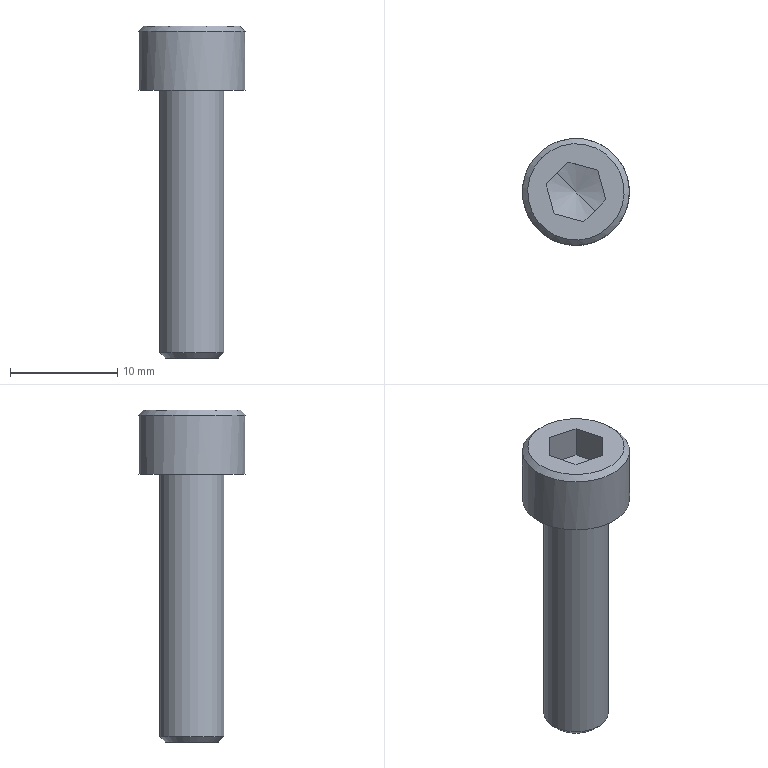Part | NX | features 1 2 | 1 solid | 21 faces | box 10 x 10 x 31 mm | volume 1098 mm3 | plane 15 | cone 4 | cylinder 2 | commonest cylinder face diameters 6 x1 10 x1
STEP:
#1=CARTESIAN_POINT('',(555.48,-112.98,-43.5));
#2=VERTEX_POINT('',#1);
#3=CARTESIAN_POINT('',(557.521,-115.021,-44.5));
#4=VERTEX_POINT('',#3);
#5=CARTESIAN_POINT('',(556.5,-114.,-44.));
#6=DIRECTION('',(0.6682,-0.6682,-0.3273));
#7=VECTOR('',#6,1000.);
#8=LINE('',#5,#7);
#9=EDGE_CURVE('',#2,#4,#8,.T.);
#10=ORIENTED_EDGE('',*,*,#9,.T.);
#11=CARTESIAN_POINT('',(559.562,-117.062,-43.5));
#12=VERTEX_POINT('',#11);
#13=CARTESIAN_POINT('',(558.541,-116.041,-44.));
#14=DIRECTION('',(0.6682,-0.6682,0.3273));
#15=VECTOR('',#14,1000.);
#16=LINE('',#13,#15);
#17=EDGE_CURVE('',#4,#12,#16,.T.);
#18=ORIENTED_EDGE('',*,*,#17,.T.);
#19=CARTESIAN_POINT('',(560.309,-115.768,-43.5));
#20=VERTEX_POINT('',#19);
#21=CARTESIAN_POINT('',(557.521,-115.021,-43.5));
#22=DIRECTION('',(0.,0.,1.));
#23=DIRECTION('',(0.7071,-0.7071,0.));
#24=AXIS2_PLACEMENT_3D('',#21,#22,#23);
#25=CIRCLE('',#24,2.887);
#26=EDGE_CURVE('',#12,#20,#25,.T.);
#27=ORIENTED_EDGE('',*,*,#26,.T.);
#28=CARTESIAN_POINT('',(559.562,-112.98,-43.5));
#29=VERTEX_POINT('',#28);
#30=CARTESIAN_POINT('',(557.521,-115.021,-43.5));
#31=DIRECTION('',(0.,0.,1.));
#32=DIRECTION('',(0.7071,-0.7071,0.));
#33=AXIS2_PLACEMENT_3D('',#30,#31,#32);
#34=CIRCLE('',#33,2.887);
#35=EDGE_CURVE('',#20,#29,#34,.T.);
#36=ORIENTED_EDGE('',*,*,#35,.T.);
#37=CARTESIAN_POINT('',(556.774,-112.232,-43.5));
#38=VERTEX_POINT('',#37);
#39=CARTESIAN_POINT('',(557.521,-115.021,-43.5));
#40=DIRECTION('',(0.,0.,1.));
#41=DIRECTION('',(0.7071,-0.7071,0.));
#42=AXIS2_PLACEMENT_3D('',#39,#40,#41);
#43=CIRCLE('',#42,2.887);
#44=EDGE_CURVE('',#29,#38,#43,.T.);
#45=ORIENTED_EDGE('',*,*,#44,.T.);
#46=CARTESIAN_POINT('',(557.521,-115.021,-43.5));
#47=DIRECTION('',(0.,0.,1.));
#48=DIRECTION('',(0.7071,-0.7071,0.));
#49=AXIS2_PLACEMENT_3D('',#46,#47,#48);
#50=CIRCLE('',#49,2.887);
#51=EDGE_CURVE('',#38,#2,#50,.T.);
#52=ORIENTED_EDGE('',*,*,#51,.T.);
#53=EDGE_LOOP('',(#10,#18,#27,#36,#45,#52));
#54=FACE_BOUND('',#53,.T.);
#55=CARTESIAN_POINT('',(557.521,-115.021,-44.));
#56=DIRECTION('',(0.,0.,1.));
#57=DIRECTION('',(-0.7071,0.7071,0.));
#58=AXIS2_PLACEMENT_3D('',#55,#56,#57);
#59=CONICAL_SURFACE('',#58,1.443,1.237);
#60=ADVANCED_FACE('',(#54),#59,.F.);
#61=CARTESIAN_POINT('',(555.399,-112.899,-71.));
#62=VERTEX_POINT('',#61);
#63=CARTESIAN_POINT('',(557.521,-115.021,-71.));
#64=DIRECTION('',(0.,0.,-1.));
#65=DIRECTION('',(-0.7071,0.7071,0.));
#66=AXIS2_PLACEMENT_3D('',#63,#64,#65);
#67=CIRCLE('',#66,3.);
#68=EDGE_CURVE('',#62,#62,#67,.T.);
#69=ORIENTED_EDGE('',*,*,#68,.T.);
#70=EDGE_LOOP('',(#69));
#71=FACE_BOUND('',#70,.T.);
#72=CARTESIAN_POINT('',(555.753,-113.253,-71.5));
#73=VERTEX_POINT('',#72);
#74=CARTESIAN_POINT('',(557.521,-115.021,-71.5));
#75=DIRECTION('',(0.,0.,1.));
#76=DIRECTION('',(-0.7071,0.7071,0.));
#77=AXIS2_PLACEMENT_3D('',#74,#75,#76);
#78=CIRCLE('',#77,2.5);
#79=EDGE_CURVE('',#73,#73,#78,.T.);
#80=ORIENTED_EDGE('',*,*,#79,.T.);
#81=EDGE_LOOP('',(#80));
#82=FACE_BOUND('',#81,.T.);
#83=CARTESIAN_POINT('',(557.521,-115.021,-71.5));
#84=DIRECTION('',(0.,0.,1.));
#85=DIRECTION('',(0.7071,-0.7071,0.));
#86=AXIS2_PLACEMENT_3D('',#83,#84,#85);
#87=CONICAL_SURFACE('',#86,2.5,0.7854);
#88=ADVANCED_FACE('',(#71,#82),#87,.T.);
#89=ORIENTED_EDGE('',*,*,#68,.F.);
#90=EDGE_LOOP('',(#89));
#91=FACE_BOUND('',#90,.T.);
#92=CARTESIAN_POINT('',(559.642,-117.142,-46.5));
#93=VERTEX_POINT('',#92);
#94=CARTESIAN_POINT('',(557.521,-115.021,-46.5));
#95=DIRECTION('',(0.,0.,1.));
#96=DIRECTION('',(0.7071,-0.7071,0.));
#97=AXIS2_PLACEMENT_3D('',#94,#95,#96);
#98=CIRCLE('',#97,3.);
#99=EDGE_CURVE('',#93,#93,#98,.T.);
#100=ORIENTED_EDGE('',*,*,#99,.F.);
#101=EDGE_LOOP('',(#100));
#102=FACE_BOUND('',#101,.T.);
#103=CARTESIAN_POINT('',(557.521,-115.021,-59.));
#104=DIRECTION('',(0.,0.,-1.));
#105=DIRECTION('',(-0.7071,0.7071,0.));
#106=AXIS2_PLACEMENT_3D('',#103,#104,#105);
#107=CYLINDRICAL_SURFACE('',#106,3.);
#108=ADVANCED_FACE('',(#91,#102),#107,.T.);
#109=ORIENTED_EDGE('',*,*,#79,.F.);
#110=EDGE_LOOP('',(#109));
#111=FACE_BOUND('',#110,.T.);
#112=CARTESIAN_POINT('',(557.521,-115.021,-71.5));
#113=DIRECTION('',(0.,0.,-1.));
#114=DIRECTION('',(-0.7071,0.7071,0.));
#115=AXIS2_PLACEMENT_3D('',#112,#113,#114);
#116=PLANE('',#115);
#117=ADVANCED_FACE('',(#111),#116,.T.);
#118=CARTESIAN_POINT('',(553.985,-111.485,-41.));
#119=VERTEX_POINT('',#118);
#120=CARTESIAN_POINT('',(557.521,-115.021,-41.));
#121=DIRECTION('',(0.,0.,1.));
#122=DIRECTION('',(-0.7071,0.7071,0.));
#123=AXIS2_PLACEMENT_3D('',#120,#121,#122);
#124=CIRCLE('',#123,5.);
#125=EDGE_CURVE('',#119,#119,#124,.T.);
#126=ORIENTED_EDGE('',*,*,#125,.T.);
#127=EDGE_LOOP('',(#126));
#128=FACE_BOUND('',#127,.T.);
#129=CARTESIAN_POINT('',(554.339,-111.839,-40.5));
#130=VERTEX_POINT('',#129);
#131=CARTESIAN_POINT('',(557.521,-115.021,-40.5));
#132=DIRECTION('',(0.,0.,-1.));
#133=DIRECTION('',(-0.7071,0.7071,0.));
#134=AXIS2_PLACEMENT_3D('',#131,#132,#133);
#135=CIRCLE('',#134,4.5);
#136=EDGE_CURVE('',#130,#130,#135,.T.);
#137=ORIENTED_EDGE('',*,*,#136,.T.);
#138=EDGE_LOOP('',(#137));
#139=FACE_BOUND('',#138,.T.);
#140=CARTESIAN_POINT('',(557.521,-115.021,-40.5));
#141=DIRECTION('',(0.,0.,-1.));
#142=DIRECTION('',(0.7071,-0.7071,0.));
#143=AXIS2_PLACEMENT_3D('',#140,#141,#142);
#144=CONICAL_SURFACE('',#143,4.5,0.7854);
#145=ADVANCED_FACE('',(#128,#139),#144,.T.);
#146=CARTESIAN_POINT('',(561.056,-118.556,-46.5));
#147=VERTEX_POINT('',#146);
#148=CARTESIAN_POINT('',(557.521,-115.021,-46.5));
#149=DIRECTION('',(0.,0.,-1.));
#150=DIRECTION('',(0.7071,-0.7071,0.));
#151=AXIS2_PLACEMENT_3D('',#148,#149,#150);
#152=CIRCLE('',#151,5.);
#153=EDGE_CURVE('',#147,#147,#152,.T.);
#154=ORIENTED_EDGE('',*,*,#153,.F.);
#155=EDGE_LOOP('',(#154));
#156=FACE_BOUND('',#155,.T.);
#157=ORIENTED_EDGE('',*,*,#125,.F.);
#158=EDGE_LOOP('',(#157));
#159=FACE_BOUND('',#158,.T.);
#160=CARTESIAN_POINT('',(557.521,-115.021,-43.5));
#161=DIRECTION('',(0.,0.,-1.));
#162=DIRECTION('',(-0.7071,0.7071,0.));
#163=AXIS2_PLACEMENT_3D('',#160,#161,#162);
#164=CYLINDRICAL_SURFACE('',#163,5.);
#165=ADVANCED_FACE('',(#156,#159),#164,.T.);
#166=CARTESIAN_POINT('',(559.562,-112.98,-40.5));
#167=VERTEX_POINT('',#166);
#168=CARTESIAN_POINT('',(560.309,-115.768,-40.5));
#169=VERTEX_POINT('',#168);
#170=CARTESIAN_POINT('',(559.936,-114.374,-40.5));
#171=DIRECTION('',(0.2588,-0.9659,0.));
#172=VECTOR('',#171,1000.);
#173=LINE('',#170,#172);
#174=EDGE_CURVE('',#167,#169,#173,.T.);
#175=ORIENTED_EDGE('',*,*,#174,.T.);
#176=CARTESIAN_POINT('',(558.268,-117.809,-40.5));
#177=VERTEX_POINT('',#176);
#178=CARTESIAN_POINT('',(559.289,-116.789,-40.5));
#179=DIRECTION('',(-0.7071,-0.7071,0.));
#180=VECTOR('',#179,1000.);
#181=LINE('',#178,#180);
#182=EDGE_CURVE('',#169,#177,#181,.T.);
#183=ORIENTED_EDGE('',*,*,#182,.T.);
#184=CARTESIAN_POINT('',(555.48,-117.062,-40.5));
#185=VERTEX_POINT('',#184);
#186=CARTESIAN_POINT('',(556.874,-117.436,-40.5));
#187=DIRECTION('',(-0.9659,0.2588,0.));
#188=VECTOR('',#187,1000.);
#189=LINE('',#186,#188);
#190=EDGE_CURVE('',#177,#185,#189,.T.);
#191=ORIENTED_EDGE('',*,*,#190,.T.);
#192=CARTESIAN_POINT('',(554.732,-114.274,-40.5));
#193=VERTEX_POINT('',#192);
#194=CARTESIAN_POINT('',(555.106,-115.668,-40.5));
#195=DIRECTION('',(-0.2588,0.9659,0.));
#196=VECTOR('',#195,1000.);
#197=LINE('',#194,#196);
#198=EDGE_CURVE('',#185,#193,#197,.T.);
#199=ORIENTED_EDGE('',*,*,#198,.T.);
#200=CARTESIAN_POINT('',(556.774,-112.232,-40.5));
#201=VERTEX_POINT('',#200);
#202=CARTESIAN_POINT('',(555.753,-113.253,-40.5));
#203=DIRECTION('',(0.7071,0.7071,0.));
#204=VECTOR('',#203,1000.);
#205=LINE('',#202,#204);
#206=EDGE_CURVE('',#193,#201,#205,.T.);
#207=ORIENTED_EDGE('',*,*,#206,.T.);
#208=CARTESIAN_POINT('',(558.168,-112.606,-40.5));
#209=DIRECTION('',(0.9659,-0.2588,0.));
#210=VECTOR('',#209,1000.);
#211=LINE('',#208,#210);
#212=EDGE_CURVE('',#201,#167,#211,.T.);
#213=ORIENTED_EDGE('',*,*,#212,.T.);
#214=EDGE_LOOP('',(#175,#183,#191,#199,#207,#213));
#215=FACE_BOUND('',#214,.T.);
#216=ORIENTED_EDGE('',*,*,#136,.F.);
#217=EDGE_LOOP('',(#216));
#218=FACE_BOUND('',#217,.T.);
#219=CARTESIAN_POINT('',(557.521,-115.021,-40.5));
#220=DIRECTION('',(0.,0.,1.));
#221=DIRECTION('',(0.7071,-0.7071,0.));
#222=AXIS2_PLACEMENT_3D('',#219,#220,#221);
#223=PLANE('',#222);
#224=ADVANCED_FACE('',(#215,#218),#223,.T.);
#225=CARTESIAN_POINT('',(559.936,-114.374,-43.5));
#226=DIRECTION('',(0.2588,-0.9659,0.));
#227=VECTOR('',#226,1000.);
#228=LINE('',#225,#227);
#229=EDGE_CURVE('',#29,#20,#228,.T.);
#230=ORIENTED_EDGE('',*,*,#229,.F.);
#231=ORIENTED_EDGE('',*,*,#35,.F.);
#232=EDGE_LOOP('',(#230,#231));
#233=FACE_BOUND('',#232,.T.);
#234=CARTESIAN_POINT('',(557.521,-115.021,-43.5));
#235=DIRECTION('',(0.,0.,1.));
#236=DIRECTION('',(0.7071,-0.7071,0.));
#237=AXIS2_PLACEMENT_3D('',#234,#235,#236);
#238=PLANE('',#237);
#239=ADVANCED_FACE('',(#233),#238,.F.);
#240=CARTESIAN_POINT('',(558.268,-117.809,-43.5));
#241=VERTEX_POINT('',#240);
#242=CARTESIAN_POINT('',(559.289,-116.789,-43.5));
#243=DIRECTION('',(-0.7071,-0.7071,0.));
#244=VECTOR('',#243,1000.);
#245=LINE('',#242,#244);
#246=EDGE_CURVE('',#20,#241,#245,.T.);
#247=ORIENTED_EDGE('',*,*,#246,.F.);
#248=ORIENTED_EDGE('',*,*,#26,.F.);
#249=CARTESIAN_POINT('',(557.521,-115.021,-43.5));
#250=DIRECTION('',(0.,0.,1.));
#251=DIRECTION('',(0.7071,-0.7071,0.));
#252=AXIS2_PLACEMENT_3D('',#249,#250,#251);
#253=CIRCLE('',#252,2.887);
#254=EDGE_CURVE('',#241,#12,#253,.T.);
#255=ORIENTED_EDGE('',*,*,#254,.F.);
#256=EDGE_LOOP('',(#247,#248,#255));
#257=FACE_BOUND('',#256,.T.);
#258=CARTESIAN_POINT('',(557.521,-115.021,-43.5));
#259=DIRECTION('',(0.,0.,1.));
#260=DIRECTION('',(0.7071,-0.7071,0.));
#261=AXIS2_PLACEMENT_3D('',#258,#259,#260);
#262=PLANE('',#261);
#263=ADVANCED_FACE('',(#257),#262,.F.);
#264=CARTESIAN_POINT('',(555.48,-117.062,-43.5));
#265=VERTEX_POINT('',#264);
#266=CARTESIAN_POINT('',(556.874,-117.436,-43.5));
#267=DIRECTION('',(-0.9659,0.2588,0.));
#268=VECTOR('',#267,1000.);
#269=LINE('',#266,#268);
#270=EDGE_CURVE('',#241,#265,#269,.T.);
#271=ORIENTED_EDGE('',*,*,#270,.F.);
#272=CARTESIAN_POINT('',(557.521,-115.021,-43.5));
#273=DIRECTION('',(0.,0.,1.));
#274=DIRECTION('',(0.7071,-0.7071,0.));
#275=AXIS2_PLACEMENT_3D('',#272,#273,#274);
#276=CIRCLE('',#275,2.887);
#277=EDGE_CURVE('',#265,#241,#276,.T.);
#278=ORIENTED_EDGE('',*,*,#277,.F.);
#279=EDGE_LOOP('',(#271,#278));
#280=FACE_BOUND('',#279,.T.);
#281=CARTESIAN_POINT('',(557.521,-115.021,-43.5));
#282=DIRECTION('',(0.,0.,1.));
#283=DIRECTION('',(0.7071,-0.7071,0.));
#284=AXIS2_PLACEMENT_3D('',#281,#282,#283);
#285=PLANE('',#284);
#286=ADVANCED_FACE('',(#280),#285,.F.);
#287=CARTESIAN_POINT('',(554.732,-114.274,-43.5));
#288=VERTEX_POINT('',#287);
#289=CARTESIAN_POINT('',(555.106,-115.668,-43.5));
#290=DIRECTION('',(-0.2588,0.9659,0.));
#291=VECTOR('',#290,1000.);
#292=LINE('',#289,#291);
#293=EDGE_CURVE('',#265,#288,#292,.T.);
#294=ORIENTED_EDGE('',*,*,#293,.F.);
#295=CARTESIAN_POINT('',(557.521,-115.021,-43.5));
#296=DIRECTION('',(0.,0.,1.));
#297=DIRECTION('',(0.7071,-0.7071,0.));
#298=AXIS2_PLACEMENT_3D('',#295,#296,#297);
#299=CIRCLE('',#298,2.887);
#300=EDGE_CURVE('',#288,#265,#299,.T.);
#301=ORIENTED_EDGE('',*,*,#300,.F.);
#302=EDGE_LOOP('',(#294,#301));
#303=FACE_BOUND('',#302,.T.);
#304=CARTESIAN_POINT('',(557.521,-115.021,-43.5));
#305=DIRECTION('',(0.,0.,1.));
#306=DIRECTION('',(0.7071,-0.7071,0.));
#307=AXIS2_PLACEMENT_3D('',#304,#305,#306);
#308=PLANE('',#307);
#309=ADVANCED_FACE('',(#303),#308,.F.);
#310=CARTESIAN_POINT('',(555.753,-113.253,-43.5));
#311=DIRECTION('',(0.7071,0.7071,0.));
#312=VECTOR('',#311,1000.);
#313=LINE('',#310,#312);
#314=EDGE_CURVE('',#288,#38,#313,.T.);
#315=ORIENTED_EDGE('',*,*,#314,.F.);
#316=CARTESIAN_POINT('',(557.521,-115.021,-43.5));
#317=DIRECTION('',(0.,0.,1.));
#318=DIRECTION('',(0.7071,-0.7071,0.));
#319=AXIS2_PLACEMENT_3D('',#316,#317,#318);
#320=CIRCLE('',#319,2.887);
#321=EDGE_CURVE('',#2,#288,#320,.T.);
#322=ORIENTED_EDGE('',*,*,#321,.F.);
#323=ORIENTED_EDGE('',*,*,#51,.F.);
#324=EDGE_LOOP('',(#315,#322,#323));
#325=FACE_BOUND('',#324,.T.);
#326=CARTESIAN_POINT('',(557.521,-115.021,-43.5));
#327=DIRECTION('',(0.,0.,1.));
#328=DIRECTION('',(0.7071,-0.7071,0.));
#329=AXIS2_PLACEMENT_3D('',#326,#327,#328);
#330=PLANE('',#329);
#331=ADVANCED_FACE('',(#325),#330,.F.);
#332=CARTESIAN_POINT('',(558.168,-112.606,-43.5));
#333=DIRECTION('',(0.9659,-0.2588,0.));
#334=VECTOR('',#333,1000.);
#335=LINE('',#332,#334);
#336=EDGE_CURVE('',#38,#29,#335,.T.);
#337=ORIENTED_EDGE('',*,*,#336,.F.);
#338=ORIENTED_EDGE('',*,*,#44,.F.);
#339=EDGE_LOOP('',(#337,#338));
#340=FACE_BOUND('',#339,.T.);
#341=CARTESIAN_POINT('',(557.521,-115.021,-43.5));
#342=DIRECTION('',(0.,0.,1.));
#343=DIRECTION('',(0.7071,-0.7071,0.));
#344=AXIS2_PLACEMENT_3D('',#341,#342,#343);
#345=PLANE('',#344);
#346=ADVANCED_FACE('',(#340),#345,.F.);
#347=ORIENTED_EDGE('',*,*,#9,.F.);
#348=ORIENTED_EDGE('',*,*,#321,.T.);
#349=ORIENTED_EDGE('',*,*,#300,.T.);
#350=ORIENTED_EDGE('',*,*,#277,.T.);
#351=ORIENTED_EDGE('',*,*,#254,.T.);
#352=ORIENTED_EDGE('',*,*,#17,.F.);
#353=EDGE_LOOP('',(#347,#348,#349,#350,#351,#352));
#354=FACE_BOUND('',#353,.T.);
#355=CARTESIAN_POINT('',(557.521,-115.021,-44.));
#356=DIRECTION('',(0.,0.,1.));
#357=DIRECTION('',(-0.7071,0.7071,0.));
#358=AXIS2_PLACEMENT_3D('',#355,#356,#357);
#359=CONICAL_SURFACE('',#358,1.443,1.237);
#360=ADVANCED_FACE('',(#354),#359,.F.);
#361=CARTESIAN_POINT('',(559.562,-112.98,-42.));
#362=DIRECTION('',(0.,0.,1.));
#363=VECTOR('',#362,1000.);
#364=LINE('',#361,#363);
#365=EDGE_CURVE('',#29,#167,#364,.T.);
#366=ORIENTED_EDGE('',*,*,#365,.F.);
#367=ORIENTED_EDGE('',*,*,#229,.T.);
#368=CARTESIAN_POINT('',(560.309,-115.768,-42.));
#369=DIRECTION('',(0.,0.,1.));
#370=VECTOR('',#369,1000.);
#371=LINE('',#368,#370);
#372=EDGE_CURVE('',#20,#169,#371,.T.);
#373=ORIENTED_EDGE('',*,*,#372,.T.);
#374=ORIENTED_EDGE('',*,*,#174,.F.);
#375=EDGE_LOOP('',(#366,#367,#373,#374));
#376=FACE_BOUND('',#375,.T.);
#377=CARTESIAN_POINT('',(559.936,-114.374,-42.));
#378=DIRECTION('',(-0.9659,-0.2588,0.));
#379=DIRECTION('',(0.,0.,1.));
#380=AXIS2_PLACEMENT_3D('',#377,#378,#379);
#381=PLANE('',#380);
#382=ADVANCED_FACE('',(#376),#381,.T.);
#383=CARTESIAN_POINT('',(556.774,-112.232,-42.));
#384=DIRECTION('',(0.,0.,1.));
#385=VECTOR('',#384,1000.);
#386=LINE('',#383,#385);
#387=EDGE_CURVE('',#38,#201,#386,.T.);
#388=ORIENTED_EDGE('',*,*,#387,.F.);
#389=ORIENTED_EDGE('',*,*,#336,.T.);
#390=ORIENTED_EDGE('',*,*,#365,.T.);
#391=ORIENTED_EDGE('',*,*,#212,.F.);
#392=EDGE_LOOP('',(#388,#389,#390,#391));
#393=FACE_BOUND('',#392,.T.);
#394=CARTESIAN_POINT('',(558.168,-112.606,-42.));
#395=DIRECTION('',(-0.2588,-0.9659,0.));
#396=DIRECTION('',(0.,0.,-1.));
#397=AXIS2_PLACEMENT_3D('',#394,#395,#396);
#398=PLANE('',#397);
#399=ADVANCED_FACE('',(#393),#398,.T.);
#400=CARTESIAN_POINT('',(554.732,-114.274,-42.));
#401=DIRECTION('',(0.,0.,1.));
#402=VECTOR('',#401,1000.);
#403=LINE('',#400,#402);
#404=EDGE_CURVE('',#288,#193,#403,.T.);
#405=ORIENTED_EDGE('',*,*,#404,.F.);
#406=ORIENTED_EDGE('',*,*,#314,.T.);
#407=ORIENTED_EDGE('',*,*,#387,.T.);
#408=ORIENTED_EDGE('',*,*,#206,.F.);
#409=EDGE_LOOP('',(#405,#406,#407,#408));
#410=FACE_BOUND('',#409,.T.);
#411=CARTESIAN_POINT('',(555.753,-113.253,-42.));
#412=DIRECTION('',(0.7071,-0.7071,0.));
#413=DIRECTION('',(0.,0.,-1.));
#414=AXIS2_PLACEMENT_3D('',#411,#412,#413);
#415=PLANE('',#414);
#416=ADVANCED_FACE('',(#410),#415,.T.);
#417=CARTESIAN_POINT('',(555.48,-117.062,-42.));
#418=DIRECTION('',(0.,0.,1.));
#419=VECTOR('',#418,1000.);
#420=LINE('',#417,#419);
#421=EDGE_CURVE('',#265,#185,#420,.T.);
#422=ORIENTED_EDGE('',*,*,#421,.F.);
#423=ORIENTED_EDGE('',*,*,#293,.T.);
#424=ORIENTED_EDGE('',*,*,#404,.T.);
#425=ORIENTED_EDGE('',*,*,#198,.F.);
#426=EDGE_LOOP('',(#422,#423,#424,#425));
#427=FACE_BOUND('',#426,.T.);
#428=CARTESIAN_POINT('',(555.106,-115.668,-42.));
#429=DIRECTION('',(0.9659,0.2588,0.));
#430=DIRECTION('',(0.,0.,-1.));
#431=AXIS2_PLACEMENT_3D('',#428,#429,#430);
#432=PLANE('',#431);
#433=ADVANCED_FACE('',(#427),#432,.T.);
#434=CARTESIAN_POINT('',(558.268,-117.809,-42.));
#435=DIRECTION('',(0.,0.,1.));
#436=VECTOR('',#435,1000.);
#437=LINE('',#434,#436);
#438=EDGE_CURVE('',#241,#177,#437,.T.);
#439=ORIENTED_EDGE('',*,*,#438,.F.);
#440=ORIENTED_EDGE('',*,*,#270,.T.);
#441=ORIENTED_EDGE('',*,*,#421,.T.);
#442=ORIENTED_EDGE('',*,*,#190,.F.);
#443=EDGE_LOOP('',(#439,#440,#441,#442));
#444=FACE_BOUND('',#443,.T.);
#445=CARTESIAN_POINT('',(556.874,-117.436,-42.));
#446=DIRECTION('',(0.2588,0.9659,0.));
#447=DIRECTION('',(0.,0.,1.));
#448=AXIS2_PLACEMENT_3D('',#445,#446,#447);
#449=PLANE('',#448);
#450=ADVANCED_FACE('',(#444),#449,.T.);
#451=ORIENTED_EDGE('',*,*,#372,.F.);
#452=ORIENTED_EDGE('',*,*,#246,.T.);
#453=ORIENTED_EDGE('',*,*,#438,.T.);
#454=ORIENTED_EDGE('',*,*,#182,.F.);
#455=EDGE_LOOP('',(#451,#452,#453,#454));
#456=FACE_BOUND('',#455,.T.);
#457=CARTESIAN_POINT('',(559.289,-116.789,-42.));
#458=DIRECTION('',(-0.7071,0.7071,0.));
#459=DIRECTION('',(0.,0.,1.));
#460=AXIS2_PLACEMENT_3D('',#457,#458,#459);
#461=PLANE('',#460);
#462=ADVANCED_FACE('',(#456),#461,.T.);
#463=ORIENTED_EDGE('',*,*,#99,.T.);
#464=EDGE_LOOP('',(#463));
#465=FACE_BOUND('',#464,.T.);
#466=ORIENTED_EDGE('',*,*,#153,.T.);
#467=EDGE_LOOP('',(#466));
#468=FACE_BOUND('',#467,.T.);
#469=CARTESIAN_POINT('',(557.521,-115.021,-46.5));
#470=DIRECTION('',(0.,0.,-1.));
#471=DIRECTION('',(-0.7071,0.7071,0.));
#472=AXIS2_PLACEMENT_3D('',#469,#470,#471);
#473=PLANE('',#472);
#474=ADVANCED_FACE('',(#465,#468),#473,.T.);
#475=CLOSED_SHELL('',(#60,#88,#108,#117,#145,#165,#224,#239,#263,#286,#309,#331,#346,#360,#382,#399,#416,#433,#450,#462,#474));
#476=MANIFOLD_SOLID_BREP('',#475);
#477=(LENGTH_UNIT()NAMED_UNIT(*)SI_UNIT(.MILLI.,.METRE.));
#478=UNCERTAINTY_MEASURE_WITH_UNIT(LENGTH_MEASURE(0.00001),#477,'','');
#479=(NAMED_UNIT(*)PLANE_ANGLE_UNIT()SI_UNIT($,.RADIAN.));
#480=(NAMED_UNIT(*)SI_UNIT($,.STERADIAN.)SOLID_ANGLE_UNIT());
#481=(GEOMETRIC_REPRESENTATION_CONTEXT(3)GLOBAL_UNCERTAINTY_ASSIGNED_CONTEXT((#478))GLOBAL_UNIT_ASSIGNED_CONTEXT((#477,#479,#480))REPRESENTATION_CONTEXT('',''));
#482=ADVANCED_BREP_SHAPE_REPRESENTATION('',(#476),#481);